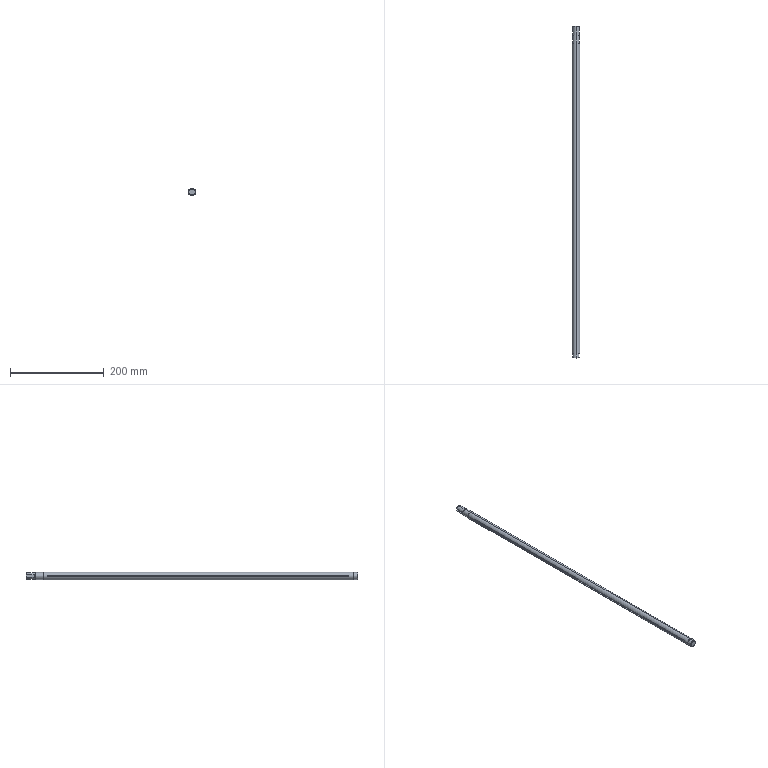Part | STEP file | PN_0001 Driving Shaft | 1 solid | 29 faces | box 16 x 710 x 16 mm | volume 135949 mm3 | cylinder 11 | plane 11 | cone 5 | spline 2 | commonest cylinder face diameters 15 x4 14 x3 5 x2 16 x2